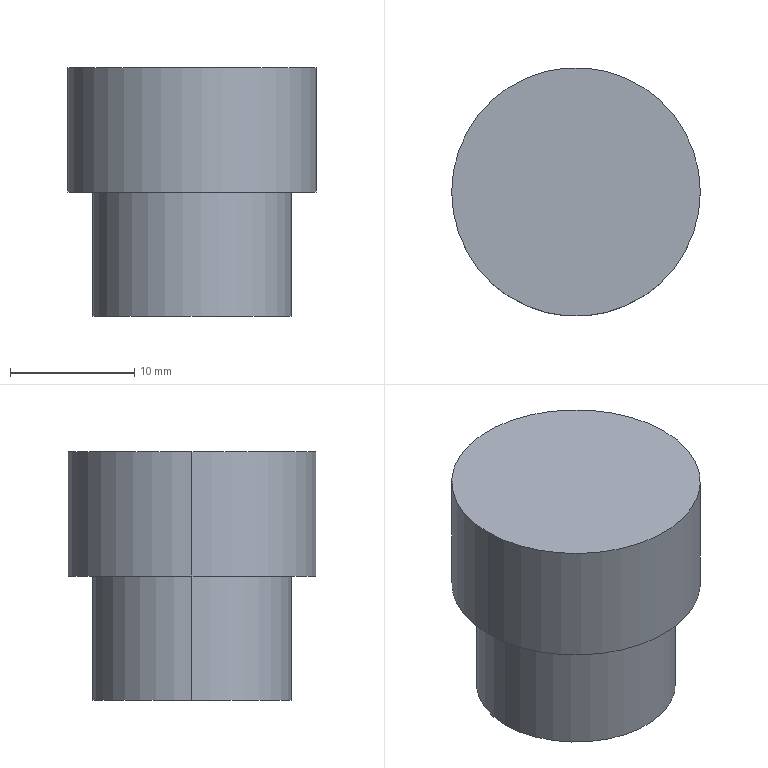Part | SolidWorks | features Extrusion 1, ICE 1 | 1 solid | 7 faces | box 20 x 20 x 20 mm | volume 5152 mm3 | cylinder 4 | plane 3 | commonest cylinder face diameters 16 x2 20 x2
STEP:
#1=CARTESIAN_POINT('',(10.,0.,10.));
#2=VERTEX_POINT('',#1);
#3=CARTESIAN_POINT('',(-10.,0.,10.));
#4=VERTEX_POINT('',#3);
#5=CARTESIAN_POINT('',(0.,0.,10.));
#6=DIRECTION('',(0.,0.,1.));
#7=DIRECTION('',(1.,0.,0.));
#8=AXIS2_PLACEMENT_3D('',#5,#6,#7);
#9=CIRCLE('',#8,10.);
#10=EDGE_CURVE('',#2,#4,#9,.T.);
#11=ORIENTED_EDGE('',*,*,#10,.F.);
#12=CARTESIAN_POINT('',(10.,0.,0.));
#13=VERTEX_POINT('',#12);
#14=CARTESIAN_POINT('',(10.,0.,10.));
#15=DIRECTION('',(0.,0.,-1.));
#16=VECTOR('',#15,1000.);
#17=LINE('',#14,#16);
#18=EDGE_CURVE('',#2,#13,#17,.T.);
#19=ORIENTED_EDGE('',*,*,#18,.T.);
#20=CARTESIAN_POINT('',(-10.,0.,0.));
#21=VERTEX_POINT('',#20);
#22=CARTESIAN_POINT('',(0.,0.,0.));
#23=DIRECTION('',(0.,0.,1.));
#24=DIRECTION('',(1.,0.,0.));
#25=AXIS2_PLACEMENT_3D('',#22,#23,#24);
#26=CIRCLE('',#25,10.);
#27=EDGE_CURVE('',#13,#21,#26,.T.);
#28=ORIENTED_EDGE('',*,*,#27,.T.);
#29=CARTESIAN_POINT('',(-10.,0.,10.));
#30=DIRECTION('',(0.,0.,-1.));
#31=VECTOR('',#30,1000.);
#32=LINE('',#29,#31);
#33=EDGE_CURVE('',#4,#21,#32,.T.);
#34=ORIENTED_EDGE('',*,*,#33,.F.);
#35=EDGE_LOOP('',(#11,#19,#28,#34));
#36=FACE_OUTER_BOUND('',#35,.T.);
#37=CARTESIAN_POINT('',(0.,0.,10.));
#38=DIRECTION('',(0.,0.,-1.));
#39=DIRECTION('',(-1.,0.,0.));
#40=AXIS2_PLACEMENT_3D('',#37,#38,#39);
#41=CYLINDRICAL_SURFACE('',#40,10.);
#42=ADVANCED_FACE('',(#36),#41,.T.);
#43=CARTESIAN_POINT('',(8.,0.,-10.));
#44=VERTEX_POINT('',#43);
#45=CARTESIAN_POINT('',(-8.,0.,-10.));
#46=VERTEX_POINT('',#45);
#47=CARTESIAN_POINT('',(0.,0.,-10.));
#48=DIRECTION('',(0.,0.,1.));
#49=DIRECTION('',(1.,0.,0.));
#50=AXIS2_PLACEMENT_3D('',#47,#48,#49);
#51=CIRCLE('',#50,8.);
#52=EDGE_CURVE('',#44,#46,#51,.T.);
#53=ORIENTED_EDGE('',*,*,#52,.T.);
#54=CARTESIAN_POINT('',(-8.,0.,0.));
#55=VERTEX_POINT('',#54);
#56=CARTESIAN_POINT('',(-8.,0.,-10.));
#57=DIRECTION('',(0.,0.,1.));
#58=VECTOR('',#57,1000.);
#59=LINE('',#56,#58);
#60=EDGE_CURVE('',#46,#55,#59,.T.);
#61=ORIENTED_EDGE('',*,*,#60,.T.);
#62=CARTESIAN_POINT('',(8.,0.,0.));
#63=VERTEX_POINT('',#62);
#64=CARTESIAN_POINT('',(0.,0.,0.));
#65=DIRECTION('',(0.,0.,1.));
#66=DIRECTION('',(1.,0.,0.));
#67=AXIS2_PLACEMENT_3D('',#64,#65,#66);
#68=CIRCLE('',#67,8.);
#69=EDGE_CURVE('',#63,#55,#68,.T.);
#70=ORIENTED_EDGE('',*,*,#69,.F.);
#71=CARTESIAN_POINT('',(8.,0.,-10.));
#72=DIRECTION('',(0.,0.,1.));
#73=VECTOR('',#72,1000.);
#74=LINE('',#71,#73);
#75=EDGE_CURVE('',#44,#63,#74,.T.);
#76=ORIENTED_EDGE('',*,*,#75,.F.);
#77=EDGE_LOOP('',(#53,#61,#70,#76));
#78=FACE_OUTER_BOUND('',#77,.T.);
#79=CARTESIAN_POINT('',(0.,0.,-10.));
#80=DIRECTION('',(0.,0.,1.));
#81=DIRECTION('',(1.,0.,0.));
#82=AXIS2_PLACEMENT_3D('',#79,#80,#81);
#83=CYLINDRICAL_SURFACE('',#82,8.);
#84=ADVANCED_FACE('',(#78),#83,.T.);
#85=ORIENTED_EDGE('',*,*,#60,.F.);
#86=CARTESIAN_POINT('',(0.,0.,-10.));
#87=DIRECTION('',(0.,0.,1.));
#88=DIRECTION('',(1.,0.,0.));
#89=AXIS2_PLACEMENT_3D('',#86,#87,#88);
#90=CIRCLE('',#89,8.);
#91=EDGE_CURVE('',#46,#44,#90,.T.);
#92=ORIENTED_EDGE('',*,*,#91,.T.);
#93=ORIENTED_EDGE('',*,*,#75,.T.);
#94=CARTESIAN_POINT('',(0.,0.,0.));
#95=DIRECTION('',(0.,0.,1.));
#96=DIRECTION('',(1.,0.,0.));
#97=AXIS2_PLACEMENT_3D('',#94,#95,#96);
#98=CIRCLE('',#97,8.);
#99=EDGE_CURVE('',#55,#63,#98,.T.);
#100=ORIENTED_EDGE('',*,*,#99,.F.);
#101=EDGE_LOOP('',(#85,#92,#93,#100));
#102=FACE_OUTER_BOUND('',#101,.T.);
#103=CARTESIAN_POINT('',(0.,0.,-10.));
#104=DIRECTION('',(0.,0.,1.));
#105=DIRECTION('',(1.,0.,0.));
#106=AXIS2_PLACEMENT_3D('',#103,#104,#105);
#107=CYLINDRICAL_SURFACE('',#106,8.);
#108=ADVANCED_FACE('',(#102),#107,.T.);
#109=ORIENTED_EDGE('',*,*,#52,.F.);
#110=ORIENTED_EDGE('',*,*,#91,.F.);
#111=EDGE_LOOP('',(#109,#110));
#112=FACE_OUTER_BOUND('',#111,.T.);
#113=CARTESIAN_POINT('',(0.,0.,-10.));
#114=DIRECTION('',(0.,0.,1.));
#115=DIRECTION('',(1.,0.,0.));
#116=AXIS2_PLACEMENT_3D('',#113,#114,#115);
#117=PLANE('',#116);
#118=ADVANCED_FACE('',(#112),#117,.F.);
#119=ORIENTED_EDGE('',*,*,#18,.F.);
#120=CARTESIAN_POINT('',(0.,0.,10.));
#121=DIRECTION('',(0.,0.,1.));
#122=DIRECTION('',(1.,0.,0.));
#123=AXIS2_PLACEMENT_3D('',#120,#121,#122);
#124=CIRCLE('',#123,10.);
#125=EDGE_CURVE('',#4,#2,#124,.T.);
#126=ORIENTED_EDGE('',*,*,#125,.F.);
#127=ORIENTED_EDGE('',*,*,#33,.T.);
#128=CARTESIAN_POINT('',(0.,0.,0.));
#129=DIRECTION('',(0.,0.,1.));
#130=DIRECTION('',(1.,0.,0.));
#131=AXIS2_PLACEMENT_3D('',#128,#129,#130);
#132=CIRCLE('',#131,10.);
#133=EDGE_CURVE('',#21,#13,#132,.T.);
#134=ORIENTED_EDGE('',*,*,#133,.T.);
#135=EDGE_LOOP('',(#119,#126,#127,#134));
#136=FACE_OUTER_BOUND('',#135,.T.);
#137=CARTESIAN_POINT('',(0.,0.,10.));
#138=DIRECTION('',(0.,0.,-1.));
#139=DIRECTION('',(-1.,0.,0.));
#140=AXIS2_PLACEMENT_3D('',#137,#138,#139);
#141=CYLINDRICAL_SURFACE('',#140,10.);
#142=ADVANCED_FACE('',(#136),#141,.T.);
#143=ORIENTED_EDGE('',*,*,#125,.T.);
#144=ORIENTED_EDGE('',*,*,#10,.T.);
#145=EDGE_LOOP('',(#143,#144));
#146=FACE_OUTER_BOUND('',#145,.T.);
#147=CARTESIAN_POINT('',(0.,0.,10.));
#148=DIRECTION('',(0.,0.,1.));
#149=DIRECTION('',(1.,0.,0.));
#150=AXIS2_PLACEMENT_3D('',#147,#148,#149);
#151=PLANE('',#150);
#152=ADVANCED_FACE('',(#146),#151,.T.);
#153=ORIENTED_EDGE('',*,*,#69,.T.);
#154=ORIENTED_EDGE('',*,*,#99,.T.);
#155=EDGE_LOOP('',(#153,#154));
#156=FACE_BOUND('',#155,.T.);
#157=ORIENTED_EDGE('',*,*,#133,.F.);
#158=ORIENTED_EDGE('',*,*,#27,.F.);
#159=EDGE_LOOP('',(#157,#158));
#160=FACE_OUTER_BOUND('',#159,.T.);
#161=CARTESIAN_POINT('',(0.,0.,0.));
#162=DIRECTION('',(0.,0.,1.));
#163=DIRECTION('',(1.,0.,0.));
#164=AXIS2_PLACEMENT_3D('',#161,#162,#163);
#165=PLANE('',#164);
#166=ADVANCED_FACE('',(#156,#160),#165,.F.);
#167=CLOSED_SHELL('',(#42,#84,#108,#118,#142,#152,#166));
#168=MANIFOLD_SOLID_BREP('',#167);
#169=CARTESIAN_POINT('',(0.,0.,0.));
#170=DIRECTION('',(0.,0.,1.));
#171=DIRECTION('',(1.,0.,0.));
#172=AXIS2_PLACEMENT_3D('',#169,#170,#171);
#173=(LENGTH_UNIT()NAMED_UNIT(*)SI_UNIT(.MILLI.,.METRE.));
#174=UNCERTAINTY_MEASURE_WITH_UNIT(LENGTH_MEASURE(0.00001),#173,'','');
#175=(NAMED_UNIT(*)PLANE_ANGLE_UNIT()SI_UNIT($,.RADIAN.));
#176=(NAMED_UNIT(*)SI_UNIT($,.STERADIAN.)SOLID_ANGLE_UNIT());
#177=(GEOMETRIC_REPRESENTATION_CONTEXT(3)GLOBAL_UNCERTAINTY_ASSIGNED_CONTEXT((#174))GLOBAL_UNIT_ASSIGNED_CONTEXT((#173,#175,#176))REPRESENTATION_CONTEXT('',''));
#178=ADVANCED_BREP_SHAPE_REPRESENTATION('',(#168,#172),#177);